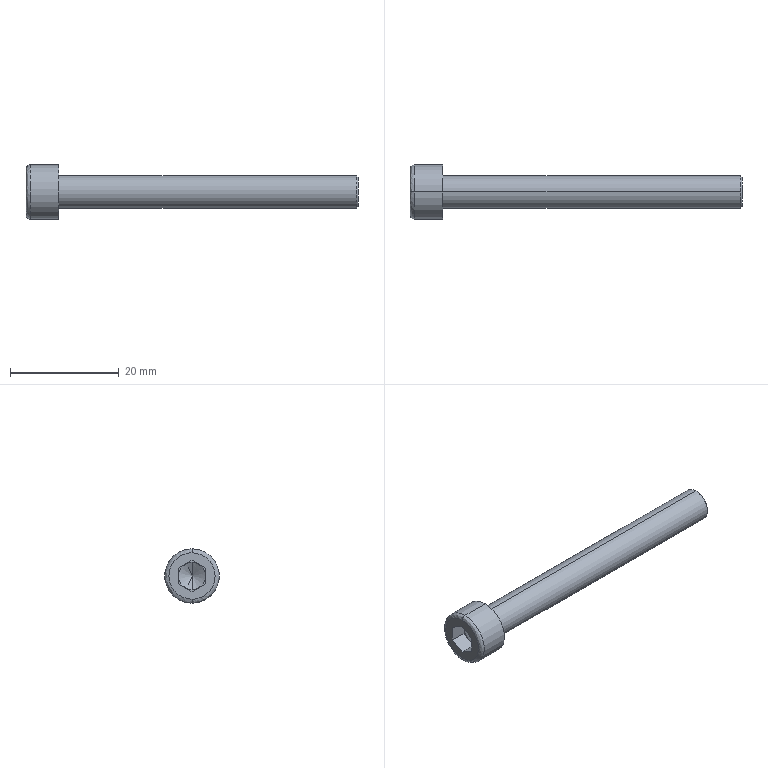Part | STEP file | hexagon socket head cap screws gb_GB_FASTENER_SCREWS_HSHCS M6X55-N | 1 solid | 25 faces | box 61 x 10 x 10 mm | volume 1948 mm3 | plane 15 | cylinder 4 | cone 4 | spline 2 | commonest cylinder face diameters 6 x2 10 x2
STEP:
#1=CARTESIAN_POINT('',(0.75,0.,5.));
#2=VERTEX_POINT('',#1);
#3=CARTESIAN_POINT('',(0.75,0.,-5.));
#4=VERTEX_POINT('',#3);
#5=CARTESIAN_POINT('',(0.75,0.,0.));
#6=DIRECTION('',(1.,0.,0.));
#7=DIRECTION('',(0.,0.,1.));
#8=AXIS2_PLACEMENT_3D('',#5,#6,#7);
#9=CIRCLE('',#8,5.);
#10=EDGE_CURVE('',#2,#4,#9,.T.);
#11=ORIENTED_EDGE('',*,*,#10,.F.);
#12=CARTESIAN_POINT('',(0.,0.,4.25));
#13=VERTEX_POINT('',#12);
#14=CARTESIAN_POINT('',(0.75,0.,4.25));
#15=DIRECTION('',(0.,-1.,0.));
#16=DIRECTION('',(0.,0.,1.));
#17=AXIS2_PLACEMENT_3D('',#14,#15,#16);
#18=CIRCLE('',#17,0.75);
#19=EDGE_CURVE('',#2,#13,#18,.T.);
#20=ORIENTED_EDGE('',*,*,#19,.T.);
#21=CARTESIAN_POINT('',(0.,0.,-4.25));
#22=VERTEX_POINT('',#21);
#23=CARTESIAN_POINT('',(0.,0.,4.25));
#24=CARTESIAN_POINT('',(0.,-8.5,4.25));
#25=CARTESIAN_POINT('',(0.,-8.5,-4.25));
#26=CARTESIAN_POINT('',(0.,0.,-4.25));
#27=(BOUNDED_CURVE()B_SPLINE_CURVE(3,(#23,#24,#25,#26),.UNSPECIFIED.,.F.,.F.)B_SPLINE_CURVE_WITH_KNOTS((4,4),(0.,1.),.UNSPECIFIED.)CURVE()GEOMETRIC_REPRESENTATION_ITEM()RATIONAL_B_SPLINE_CURVE((1.,0.3333,0.3333,1.))REPRESENTATION_ITEM(''));
#28=EDGE_CURVE('',#13,#22,#27,.T.);
#29=ORIENTED_EDGE('',*,*,#28,.T.);
#30=CARTESIAN_POINT('',(0.75,0.,-4.25));
#31=DIRECTION('',(0.,1.,0.));
#32=DIRECTION('',(0.,0.,-1.));
#33=AXIS2_PLACEMENT_3D('',#30,#31,#32);
#34=CIRCLE('',#33,0.75);
#35=EDGE_CURVE('',#4,#22,#34,.T.);
#36=ORIENTED_EDGE('',*,*,#35,.F.);
#37=EDGE_LOOP('',(#11,#20,#29,#36));
#38=FACE_OUTER_BOUND('',#37,.T.);
#39=CARTESIAN_POINT('',(0.75,0.,5.));
#40=CARTESIAN_POINT('',(0.75,-10.,5.));
#41=CARTESIAN_POINT('',(0.75,-10.,-5.));
#42=CARTESIAN_POINT('',(0.75,0.,-5.));
#43=CARTESIAN_POINT('',(0.3107,0.,5.));
#44=CARTESIAN_POINT('',(0.3107,-10.,5.));
#45=CARTESIAN_POINT('',(0.3107,-10.,-5.));
#46=CARTESIAN_POINT('',(0.3107,0.,-5.));
#47=CARTESIAN_POINT('',(0.,0.,4.689));
#48=CARTESIAN_POINT('',(0.,-9.379,4.689));
#49=CARTESIAN_POINT('',(0.,-9.379,-4.689));
#50=CARTESIAN_POINT('',(0.,0.,-4.689));
#51=CARTESIAN_POINT('',(0.,0.,4.25));
#52=CARTESIAN_POINT('',(0.,-8.5,4.25));
#53=CARTESIAN_POINT('',(0.,-8.5,-4.25));
#54=CARTESIAN_POINT('',(0.,0.,-4.25));
#55=(BOUNDED_SURFACE()B_SPLINE_SURFACE(3,3,((#39,#40,#41,#42),(#43,#44,#45,#46),(#47,#48,#49,#50),(#51,#52,#53,#54)),.UNSPECIFIED.,.F.,.F.,.F.)B_SPLINE_SURFACE_WITH_KNOTS((4,4),(4,4),(0.,1.),(0.,1.),.UNSPECIFIED.)GEOMETRIC_REPRESENTATION_ITEM()RATIONAL_B_SPLINE_SURFACE(((1.,0.3333,0.3333,1.),(0.8047,0.2682,0.2682,0.8047),(0.8047,0.2682,0.2682,0.8047),(1.,0.3333,0.3333,1.)))REPRESENTATION_ITEM('')SURFACE());
#56=ADVANCED_FACE('',(#38),#55,.T.);
#57=CARTESIAN_POINT('',(60.75,0.,3.));
#58=VERTEX_POINT('',#57);
#59=CARTESIAN_POINT('',(60.75,0.,-3.));
#60=VERTEX_POINT('',#59);
#61=CARTESIAN_POINT('',(60.75,0.,0.));
#62=DIRECTION('',(-1.,0.,0.));
#63=DIRECTION('',(0.,0.,1.));
#64=AXIS2_PLACEMENT_3D('',#61,#62,#63);
#65=CIRCLE('',#64,3.);
#66=EDGE_CURVE('',#58,#60,#65,.T.);
#67=ORIENTED_EDGE('',*,*,#66,.T.);
#68=CARTESIAN_POINT('',(6.,0.,-3.));
#69=VERTEX_POINT('',#68);
#70=CARTESIAN_POINT('',(61.,0.,-3.));
#71=DIRECTION('',(-1.,0.,0.));
#72=VECTOR('',#71,1000.);
#73=LINE('',#70,#72);
#74=EDGE_CURVE('',#60,#69,#73,.T.);
#75=ORIENTED_EDGE('',*,*,#74,.T.);
#76=CARTESIAN_POINT('',(6.,0.,3.));
#77=VERTEX_POINT('',#76);
#78=CARTESIAN_POINT('',(6.,0.,0.));
#79=DIRECTION('',(1.,0.,0.));
#80=DIRECTION('',(0.,0.,1.));
#81=AXIS2_PLACEMENT_3D('',#78,#79,#80);
#82=CIRCLE('',#81,3.);
#83=EDGE_CURVE('',#69,#77,#82,.T.);
#84=ORIENTED_EDGE('',*,*,#83,.T.);
#85=CARTESIAN_POINT('',(61.,0.,3.));
#86=DIRECTION('',(-1.,0.,0.));
#87=VECTOR('',#86,1000.);
#88=LINE('',#85,#87);
#89=EDGE_CURVE('',#58,#77,#88,.T.);
#90=ORIENTED_EDGE('',*,*,#89,.F.);
#91=EDGE_LOOP('',(#67,#75,#84,#90));
#92=FACE_OUTER_BOUND('',#91,.T.);
#93=CARTESIAN_POINT('',(61.,0.,0.));
#94=DIRECTION('',(-1.,0.,0.));
#95=DIRECTION('',(0.,0.,1.));
#96=AXIS2_PLACEMENT_3D('',#93,#94,#95);
#97=CYLINDRICAL_SURFACE('',#96,3.);
#98=ADVANCED_FACE('',(#92),#97,.T.);
#99=CARTESIAN_POINT('',(61.,0.,2.75));
#100=VERTEX_POINT('',#99);
#101=CARTESIAN_POINT('',(61.,0.,-2.75));
#102=VERTEX_POINT('',#101);
#103=CARTESIAN_POINT('',(61.,0.,0.));
#104=DIRECTION('',(-1.,0.,0.));
#105=DIRECTION('',(0.,0.,1.));
#106=AXIS2_PLACEMENT_3D('',#103,#104,#105);
#107=CIRCLE('',#106,2.75);
#108=EDGE_CURVE('',#100,#102,#107,.T.);
#109=ORIENTED_EDGE('',*,*,#108,.T.);
#110=CARTESIAN_POINT('',(60.75,0.,-3.));
#111=DIRECTION('',(-0.7071,0.,-0.7071));
#112=VECTOR('',#111,1000.);
#113=LINE('',#110,#112);
#114=EDGE_CURVE('',#102,#60,#113,.T.);
#115=ORIENTED_EDGE('',*,*,#114,.T.);
#116=ORIENTED_EDGE('',*,*,#66,.F.);
#117=CARTESIAN_POINT('',(60.75,0.,3.));
#118=DIRECTION('',(-0.7071,0.,0.7071));
#119=VECTOR('',#118,1000.);
#120=LINE('',#117,#119);
#121=EDGE_CURVE('',#100,#58,#120,.T.);
#122=ORIENTED_EDGE('',*,*,#121,.F.);
#123=EDGE_LOOP('',(#109,#115,#116,#122));
#124=FACE_OUTER_BOUND('',#123,.T.);
#125=CARTESIAN_POINT('',(60.75,0.,0.));
#126=DIRECTION('',(-1.,0.,0.));
#127=DIRECTION('',(0.,0.,1.));
#128=AXIS2_PLACEMENT_3D('',#125,#126,#127);
#129=CONICAL_SURFACE('',#128,3.,0.7854);
#130=ADVANCED_FACE('',(#124),#129,.T.);
#131=CARTESIAN_POINT('',(6.,0.,-5.));
#132=VERTEX_POINT('',#131);
#133=CARTESIAN_POINT('',(6.,0.,5.));
#134=VERTEX_POINT('',#133);
#135=CARTESIAN_POINT('',(6.,0.,0.));
#136=DIRECTION('',(1.,0.,0.));
#137=DIRECTION('',(0.,0.,1.));
#138=AXIS2_PLACEMENT_3D('',#135,#136,#137);
#139=CIRCLE('',#138,5.);
#140=EDGE_CURVE('',#132,#134,#139,.T.);
#141=ORIENTED_EDGE('',*,*,#140,.F.);
#142=CARTESIAN_POINT('',(6.,0.,-5.));
#143=DIRECTION('',(-1.,0.,0.));
#144=VECTOR('',#143,1000.);
#145=LINE('',#142,#144);
#146=EDGE_CURVE('',#132,#4,#145,.T.);
#147=ORIENTED_EDGE('',*,*,#146,.T.);
#148=CARTESIAN_POINT('',(0.75,0.,0.));
#149=DIRECTION('',(1.,0.,0.));
#150=DIRECTION('',(0.,0.,1.));
#151=AXIS2_PLACEMENT_3D('',#148,#149,#150);
#152=CIRCLE('',#151,5.);
#153=EDGE_CURVE('',#4,#2,#152,.T.);
#154=ORIENTED_EDGE('',*,*,#153,.T.);
#155=CARTESIAN_POINT('',(6.,0.,5.));
#156=DIRECTION('',(-1.,0.,0.));
#157=VECTOR('',#156,1000.);
#158=LINE('',#155,#157);
#159=EDGE_CURVE('',#134,#2,#158,.T.);
#160=ORIENTED_EDGE('',*,*,#159,.F.);
#161=EDGE_LOOP('',(#141,#147,#154,#160));
#162=FACE_OUTER_BOUND('',#161,.T.);
#163=CARTESIAN_POINT('',(6.,0.,0.));
#164=DIRECTION('',(-1.,0.,0.));
#165=DIRECTION('',(0.,0.,1.));
#166=AXIS2_PLACEMENT_3D('',#163,#164,#165);
#167=CYLINDRICAL_SURFACE('',#166,5.);
#168=ADVANCED_FACE('',(#162),#167,.T.);
#169=CARTESIAN_POINT('',(4.443,0.,0.));
#170=VERTEX_POINT('',#169);
#171=CARTESIAN_POINT('',(3.,0.,2.5));
#172=VERTEX_POINT('',#171);
#173=CARTESIAN_POINT('',(3.,0.,2.5));
#174=DIRECTION('',(-0.5,0.,0.866));
#175=VECTOR('',#174,1000.);
#176=LINE('',#173,#175);
#177=EDGE_CURVE('',#170,#172,#176,.T.);
#178=ORIENTED_EDGE('',*,*,#177,.F.);
#179=CARTESIAN_POINT('',(3.,0.,-2.5));
#180=VERTEX_POINT('',#179);
#181=CARTESIAN_POINT('',(3.,0.,-2.5));
#182=DIRECTION('',(-0.5,0.,-0.866));
#183=VECTOR('',#182,1000.);
#184=LINE('',#181,#183);
#185=EDGE_CURVE('',#170,#180,#184,.T.);
#186=ORIENTED_EDGE('',*,*,#185,.T.);
#187=CARTESIAN_POINT('',(3.,-1.25,-2.165));
#188=VERTEX_POINT('',#187);
#189=CARTESIAN_POINT('',(3.,0.,0.));
#190=DIRECTION('',(1.,0.,0.));
#191=DIRECTION('',(0.,0.,1.));
#192=AXIS2_PLACEMENT_3D('',#189,#190,#191);
#193=CIRCLE('',#192,2.5);
#194=EDGE_CURVE('',#188,#180,#193,.T.);
#195=ORIENTED_EDGE('',*,*,#194,.F.);
#196=CARTESIAN_POINT('',(3.,-2.5,0.));
#197=VERTEX_POINT('',#196);
#198=CARTESIAN_POINT('',(3.,0.,0.));
#199=DIRECTION('',(1.,0.,0.));
#200=DIRECTION('',(0.,0.,1.));
#201=AXIS2_PLACEMENT_3D('',#198,#199,#200);
#202=CIRCLE('',#201,2.5);
#203=EDGE_CURVE('',#197,#188,#202,.T.);
#204=ORIENTED_EDGE('',*,*,#203,.F.);
#205=CARTESIAN_POINT('',(3.,-1.25,2.165));
#206=VERTEX_POINT('',#205);
#207=CARTESIAN_POINT('',(3.,0.,0.));
#208=DIRECTION('',(-1.,0.,0.));
#209=DIRECTION('',(0.,0.,1.));
#210=AXIS2_PLACEMENT_3D('',#207,#208,#209);
#211=CIRCLE('',#210,2.5);
#212=EDGE_CURVE('',#197,#206,#211,.T.);
#213=ORIENTED_EDGE('',*,*,#212,.T.);
#214=CARTESIAN_POINT('',(3.,0.,0.));
#215=DIRECTION('',(1.,0.,0.));
#216=DIRECTION('',(0.,0.,1.));
#217=AXIS2_PLACEMENT_3D('',#214,#215,#216);
#218=CIRCLE('',#217,2.5);
#219=EDGE_CURVE('',#172,#206,#218,.T.);
#220=ORIENTED_EDGE('',*,*,#219,.F.);
#221=EDGE_LOOP('',(#178,#186,#195,#204,#213,#220));
#222=FACE_OUTER_BOUND('',#221,.T.);
#223=CARTESIAN_POINT('',(3.,0.,0.));
#224=DIRECTION('',(-1.,0.,0.));
#225=DIRECTION('',(0.,0.,1.));
#226=AXIS2_PLACEMENT_3D('',#223,#224,#225);
#227=CONICAL_SURFACE('',#226,2.5,1.047);
#228=ADVANCED_FACE('',(#222),#227,.F.);
#229=ORIENTED_EDGE('',*,*,#74,.F.);
#230=CARTESIAN_POINT('',(60.75,0.,0.));
#231=DIRECTION('',(-1.,0.,0.));
#232=DIRECTION('',(0.,0.,1.));
#233=AXIS2_PLACEMENT_3D('',#230,#231,#232);
#234=CIRCLE('',#233,3.);
#235=EDGE_CURVE('',#60,#58,#234,.T.);
#236=ORIENTED_EDGE('',*,*,#235,.T.);
#237=ORIENTED_EDGE('',*,*,#89,.T.);
#238=CARTESIAN_POINT('',(6.,0.,0.));
#239=DIRECTION('',(1.,0.,0.));
#240=DIRECTION('',(0.,0.,1.));
#241=AXIS2_PLACEMENT_3D('',#238,#239,#240);
#242=CIRCLE('',#241,3.);
#243=EDGE_CURVE('',#77,#69,#242,.T.);
#244=ORIENTED_EDGE('',*,*,#243,.T.);
#245=EDGE_LOOP('',(#229,#236,#237,#244));
#246=FACE_OUTER_BOUND('',#245,.T.);
#247=CARTESIAN_POINT('',(61.,0.,0.));
#248=DIRECTION('',(-1.,0.,0.));
#249=DIRECTION('',(0.,0.,1.));
#250=AXIS2_PLACEMENT_3D('',#247,#248,#249);
#251=CYLINDRICAL_SURFACE('',#250,3.);
#252=ADVANCED_FACE('',(#246),#251,.T.);
#253=ORIENTED_EDGE('',*,*,#243,.F.);
#254=ORIENTED_EDGE('',*,*,#83,.F.);
#255=EDGE_LOOP('',(#253,#254));
#256=FACE_BOUND('',#255,.T.);
#257=CARTESIAN_POINT('',(6.,0.,0.));
#258=DIRECTION('',(1.,0.,0.));
#259=DIRECTION('',(0.,0.,1.));
#260=AXIS2_PLACEMENT_3D('',#257,#258,#259);
#261=CIRCLE('',#260,5.);
#262=EDGE_CURVE('',#134,#132,#261,.T.);
#263=ORIENTED_EDGE('',*,*,#262,.T.);
#264=ORIENTED_EDGE('',*,*,#140,.T.);
#265=EDGE_LOOP('',(#263,#264));
#266=FACE_OUTER_BOUND('',#265,.T.);
#267=CARTESIAN_POINT('',(6.,0.,0.));
#268=DIRECTION('',(1.,0.,0.));
#269=DIRECTION('',(0.,0.,-1.));
#270=AXIS2_PLACEMENT_3D('',#267,#268,#269);
#271=PLANE('',#270);
#272=ADVANCED_FACE('',(#256,#266),#271,.T.);
#273=ORIENTED_EDGE('',*,*,#114,.F.);
#274=CARTESIAN_POINT('',(61.,0.,0.));
#275=DIRECTION('',(-1.,0.,0.));
#276=DIRECTION('',(0.,0.,1.));
#277=AXIS2_PLACEMENT_3D('',#274,#275,#276);
#278=CIRCLE('',#277,2.75);
#279=EDGE_CURVE('',#102,#100,#278,.T.);
#280=ORIENTED_EDGE('',*,*,#279,.T.);
#281=ORIENTED_EDGE('',*,*,#121,.T.);
#282=ORIENTED_EDGE('',*,*,#235,.F.);
#283=EDGE_LOOP('',(#273,#280,#281,#282));
#284=FACE_OUTER_BOUND('',#283,.T.);
#285=CARTESIAN_POINT('',(60.75,0.,0.));
#286=DIRECTION('',(-1.,0.,0.));
#287=DIRECTION('',(0.,0.,1.));
#288=AXIS2_PLACEMENT_3D('',#285,#286,#287);
#289=CONICAL_SURFACE('',#288,3.,0.7854);
#290=ADVANCED_FACE('',(#284),#289,.T.);
#291=ORIENTED_EDGE('',*,*,#146,.F.);
#292=ORIENTED_EDGE('',*,*,#262,.F.);
#293=ORIENTED_EDGE('',*,*,#159,.T.);
#294=ORIENTED_EDGE('',*,*,#10,.T.);
#295=EDGE_LOOP('',(#291,#292,#293,#294));
#296=FACE_OUTER_BOUND('',#295,.T.);
#297=CARTESIAN_POINT('',(6.,0.,0.));
#298=DIRECTION('',(-1.,0.,0.));
#299=DIRECTION('',(0.,0.,1.));
#300=AXIS2_PLACEMENT_3D('',#297,#298,#299);
#301=CYLINDRICAL_SURFACE('',#300,5.);
#302=ADVANCED_FACE('',(#296),#301,.T.);
#303=ORIENTED_EDGE('',*,*,#108,.F.);
#304=ORIENTED_EDGE('',*,*,#279,.F.);
#305=EDGE_LOOP('',(#303,#304));
#306=FACE_OUTER_BOUND('',#305,.T.);
#307=CARTESIAN_POINT('',(61.,0.,0.));
#308=DIRECTION('',(1.,0.,0.));
#309=DIRECTION('',(0.,0.,-1.));
#310=AXIS2_PLACEMENT_3D('',#307,#308,#309);
#311=PLANE('',#310);
#312=ADVANCED_FACE('',(#306),#311,.T.);
#313=ORIENTED_EDGE('',*,*,#19,.F.);
#314=ORIENTED_EDGE('',*,*,#153,.F.);
#315=ORIENTED_EDGE('',*,*,#35,.T.);
#316=CARTESIAN_POINT('',(0.,0.,-4.25));
#317=CARTESIAN_POINT('',(0.,8.5,-4.25));
#318=CARTESIAN_POINT('',(0.,8.5,4.25));
#319=CARTESIAN_POINT('',(0.,0.,4.25));
#320=(BOUNDED_CURVE()B_SPLINE_CURVE(3,(#316,#317,#318,#319),.UNSPECIFIED.,.F.,.T.)B_SPLINE_CURVE_WITH_KNOTS((4,4),(0.,1.),.UNSPECIFIED.)CURVE()GEOMETRIC_REPRESENTATION_ITEM()RATIONAL_B_SPLINE_CURVE((1.,0.3333,0.3333,1.))REPRESENTATION_ITEM(''));
#321=EDGE_CURVE('',#22,#13,#320,.T.);
#322=ORIENTED_EDGE('',*,*,#321,.T.);
#323=EDGE_LOOP('',(#313,#314,#315,#322));
#324=FACE_OUTER_BOUND('',#323,.T.);
#325=CARTESIAN_POINT('',(0.75,0.,-5.));
#326=CARTESIAN_POINT('',(0.75,10.,-5.));
#327=CARTESIAN_POINT('',(0.75,10.,5.));
#328=CARTESIAN_POINT('',(0.75,0.,5.));
#329=CARTESIAN_POINT('',(0.3107,0.,-5.));
#330=CARTESIAN_POINT('',(0.3107,10.,-5.));
#331=CARTESIAN_POINT('',(0.3107,10.,5.));
#332=CARTESIAN_POINT('',(0.3107,0.,5.));
#333=CARTESIAN_POINT('',(0.,0.,-4.689));
#334=CARTESIAN_POINT('',(0.,9.379,-4.689));
#335=CARTESIAN_POINT('',(0.,9.379,4.689));
#336=CARTESIAN_POINT('',(0.,0.,4.689));
#337=CARTESIAN_POINT('',(0.,0.,-4.25));
#338=CARTESIAN_POINT('',(0.,8.5,-4.25));
#339=CARTESIAN_POINT('',(0.,8.5,4.25));
#340=CARTESIAN_POINT('',(0.,0.,4.25));
#341=(BOUNDED_SURFACE()B_SPLINE_SURFACE(3,3,((#325,#326,#327,#328),(#329,#330,#331,#332),(#333,#334,#335,#336),(#337,#338,#339,#340)),.UNSPECIFIED.,.F.,.F.,.F.)B_SPLINE_SURFACE_WITH_KNOTS((4,4),(4,4),(0.,1.),(0.,1.),.UNSPECIFIED.)GEOMETRIC_REPRESENTATION_ITEM()RATIONAL_B_SPLINE_SURFACE(((1.,0.3333,0.3333,1.),(0.8047,0.2682,0.2682,0.8047),(0.8047,0.2682,0.2682,0.8047),(1.,0.3333,0.3333,1.)))REPRESENTATION_ITEM('')SURFACE());
#342=ADVANCED_FACE('',(#324),#341,.T.);
#343=CARTESIAN_POINT('',(0.,2.5,-1.443));
#344=VERTEX_POINT('',#343);
#345=CARTESIAN_POINT('',(0.,0.,-2.887));
#346=VERTEX_POINT('',#345);
#347=CARTESIAN_POINT('',(0.,2.5,-1.443));
#348=DIRECTION('',(0.,-0.866,-0.5));
#349=VECTOR('',#348,1000.);
#350=LINE('',#347,#349);
#351=EDGE_CURVE('',#344,#346,#350,.T.);
#352=ORIENTED_EDGE('',*,*,#351,.F.);
#353=CARTESIAN_POINT('',(0.,2.5,1.443));
#354=VERTEX_POINT('',#353);
#355=CARTESIAN_POINT('',(0.,2.5,0.));
#356=DIRECTION('',(0.,0.,-1.));
#357=VECTOR('',#356,1000.);
#358=LINE('',#355,#357);
#359=EDGE_CURVE('',#354,#344,#358,.T.);
#360=ORIENTED_EDGE('',*,*,#359,.F.);
#361=CARTESIAN_POINT('',(0.,0.,2.887));
#362=VERTEX_POINT('',#361);
#363=CARTESIAN_POINT('',(0.,0.,2.887));
#364=DIRECTION('',(0.,0.866,-0.5));
#365=VECTOR('',#364,1000.);
#366=LINE('',#363,#365);
#367=EDGE_CURVE('',#362,#354,#366,.T.);
#368=ORIENTED_EDGE('',*,*,#367,.F.);
#369=CARTESIAN_POINT('',(0.,-2.5,1.443));
#370=VERTEX_POINT('',#369);
#371=CARTESIAN_POINT('',(0.,-2.5,1.443));
#372=DIRECTION('',(0.,0.866,0.5));
#373=VECTOR('',#372,1000.);
#374=LINE('',#371,#373);
#375=EDGE_CURVE('',#370,#362,#374,.T.);
#376=ORIENTED_EDGE('',*,*,#375,.F.);
#377=CARTESIAN_POINT('',(0.,-2.5,-1.443));
#378=VERTEX_POINT('',#377);
#379=CARTESIAN_POINT('',(0.,-2.5,0.));
#380=DIRECTION('',(0.,0.,1.));
#381=VECTOR('',#380,1000.);
#382=LINE('',#379,#381);
#383=EDGE_CURVE('',#378,#370,#382,.T.);
#384=ORIENTED_EDGE('',*,*,#383,.F.);
#385=CARTESIAN_POINT('',(0.,0.,-2.887));
#386=DIRECTION('',(0.,-0.866,0.5));
#387=VECTOR('',#386,1000.);
#388=LINE('',#385,#387);
#389=EDGE_CURVE('',#346,#378,#388,.T.);
#390=ORIENTED_EDGE('',*,*,#389,.F.);
#391=EDGE_LOOP('',(#352,#360,#368,#376,#384,#390));
#392=FACE_BOUND('',#391,.T.);
#393=ORIENTED_EDGE('',*,*,#321,.F.);
#394=ORIENTED_EDGE('',*,*,#28,.F.);
#395=EDGE_LOOP('',(#393,#394));
#396=FACE_OUTER_BOUND('',#395,.T.);
#397=CARTESIAN_POINT('',(0.,0.,0.));
#398=DIRECTION('',(1.,0.,0.));
#399=DIRECTION('',(0.,0.,-1.));
#400=AXIS2_PLACEMENT_3D('',#397,#398,#399);
#401=PLANE('',#400);
#402=ADVANCED_FACE('',(#392,#396),#401,.F.);
#403=CARTESIAN_POINT('',(3.,0.,-2.887));
#404=VERTEX_POINT('',#403);
#405=CARTESIAN_POINT('',(3.,-2.5,-1.443));
#406=DIRECTION('',(0.,0.866,-0.5));
#407=VECTOR('',#406,1000.);
#408=LINE('',#405,#407);
#409=EDGE_CURVE('',#188,#404,#408,.T.);
#410=ORIENTED_EDGE('',*,*,#409,.T.);
#411=CARTESIAN_POINT('',(3.,0.,-2.887));
#412=DIRECTION('',(-1.,0.,0.));
#413=VECTOR('',#412,1000.);
#414=LINE('',#411,#413);
#415=EDGE_CURVE('',#404,#346,#414,.T.);
#416=ORIENTED_EDGE('',*,*,#415,.T.);
#417=ORIENTED_EDGE('',*,*,#389,.T.);
#418=CARTESIAN_POINT('',(3.,-2.5,-1.443));
#419=VERTEX_POINT('',#418);
#420=CARTESIAN_POINT('',(3.,-2.5,-1.443));
#421=DIRECTION('',(1.,0.,0.));
#422=VECTOR('',#421,1000.);
#423=LINE('',#420,#422);
#424=EDGE_CURVE('',#378,#419,#423,.T.);
#425=ORIENTED_EDGE('',*,*,#424,.T.);
#426=CARTESIAN_POINT('',(3.,-2.5,-1.443));
#427=DIRECTION('',(0.,0.866,-0.5));
#428=VECTOR('',#427,1000.);
#429=LINE('',#426,#428);
#430=EDGE_CURVE('',#419,#188,#429,.T.);
#431=ORIENTED_EDGE('',*,*,#430,.T.);
#432=EDGE_LOOP('',(#410,#416,#417,#425,#431));
#433=FACE_OUTER_BOUND('',#432,.T.);
#434=CARTESIAN_POINT('',(3.,-2.5,-1.443));
#435=DIRECTION('',(0.,0.5,0.866));
#436=DIRECTION('',(0.,-0.866,0.5));
#437=AXIS2_PLACEMENT_3D('',#434,#435,#436);
#438=PLANE('',#437);
#439=ADVANCED_FACE('',(#433),#438,.T.);
#440=CARTESIAN_POINT('',(3.,1.25,-2.165));
#441=VERTEX_POINT('',#440);
#442=CARTESIAN_POINT('',(3.,2.5,-1.443));
#443=VERTEX_POINT('',#442);
#444=CARTESIAN_POINT('',(3.,1.25,-2.165));
#445=DIRECTION('',(0.,0.866,0.5));
#446=VECTOR('',#445,1000.);
#447=LINE('',#444,#446);
#448=EDGE_CURVE('',#441,#443,#447,.T.);
#449=ORIENTED_EDGE('',*,*,#448,.T.);
#450=CARTESIAN_POINT('',(3.,2.5,-1.443));
#451=DIRECTION('',(-1.,0.,0.));
#452=VECTOR('',#451,1000.);
#453=LINE('',#450,#452);
#454=EDGE_CURVE('',#443,#344,#453,.T.);
#455=ORIENTED_EDGE('',*,*,#454,.T.);
#456=ORIENTED_EDGE('',*,*,#351,.T.);
#457=ORIENTED_EDGE('',*,*,#415,.F.);
#458=CARTESIAN_POINT('',(3.,0.,-2.887));
#459=DIRECTION('',(0.,0.866,0.5));
#460=VECTOR('',#459,1000.);
#461=LINE('',#458,#460);
#462=EDGE_CURVE('',#404,#441,#461,.T.);
#463=ORIENTED_EDGE('',*,*,#462,.T.);
#464=EDGE_LOOP('',(#449,#455,#456,#457,#463));
#465=FACE_OUTER_BOUND('',#464,.T.);
#466=CARTESIAN_POINT('',(3.,0.,-2.887));
#467=DIRECTION('',(0.,-0.5,0.866));
#468=DIRECTION('',(0.,-0.866,-0.5));
#469=AXIS2_PLACEMENT_3D('',#466,#467,#468);
#470=PLANE('',#469);
#471=ADVANCED_FACE('',(#465),#470,.T.);
#472=CARTESIAN_POINT('',(3.,2.5,0.));
#473=VERTEX_POINT('',#472);
#474=CARTESIAN_POINT('',(3.,2.5,1.443));
#475=VERTEX_POINT('',#474);
#476=CARTESIAN_POINT('',(3.,2.5,-2.887));
#477=DIRECTION('',(0.,0.,1.));
#478=VECTOR('',#477,1000.);
#479=LINE('',#476,#478);
#480=EDGE_CURVE('',#473,#475,#479,.T.);
#481=ORIENTED_EDGE('',*,*,#480,.T.);
#482=CARTESIAN_POINT('',(3.,2.5,1.443));
#483=DIRECTION('',(-1.,0.,0.));
#484=VECTOR('',#483,1000.);
#485=LINE('',#482,#484);
#486=EDGE_CURVE('',#475,#354,#485,.T.);
#487=ORIENTED_EDGE('',*,*,#486,.T.);
#488=ORIENTED_EDGE('',*,*,#359,.T.);
#489=ORIENTED_EDGE('',*,*,#454,.F.);
#490=CARTESIAN_POINT('',(3.,2.5,-2.887));
#491=DIRECTION('',(0.,0.,1.));
#492=VECTOR('',#491,1000.);
#493=LINE('',#490,#492);
#494=EDGE_CURVE('',#443,#473,#493,.T.);
#495=ORIENTED_EDGE('',*,*,#494,.T.);
#496=EDGE_LOOP('',(#481,#487,#488,#489,#495));
#497=FACE_OUTER_BOUND('',#496,.T.);
#498=CARTESIAN_POINT('',(3.,2.5,-1.443));
#499=DIRECTION('',(0.,-1.,0.));
#500=DIRECTION('',(0.,0.,-1.));
#501=AXIS2_PLACEMENT_3D('',#498,#499,#500);
#502=PLANE('',#501);
#503=ADVANCED_FACE('',(#497),#502,.T.);
#504=CARTESIAN_POINT('',(3.,1.25,2.165));
#505=VERTEX_POINT('',#504);
#506=CARTESIAN_POINT('',(3.,0.,2.887));
#507=VERTEX_POINT('',#506);
#508=CARTESIAN_POINT('',(3.,2.5,1.443));
#509=DIRECTION('',(0.,-0.866,0.5));
#510=VECTOR('',#509,1000.);
#511=LINE('',#508,#510);
#512=EDGE_CURVE('',#505,#507,#511,.T.);
#513=ORIENTED_EDGE('',*,*,#512,.T.);
#514=CARTESIAN_POINT('',(3.,0.,2.887));
#515=DIRECTION('',(-1.,0.,0.));
#516=VECTOR('',#515,1000.);
#517=LINE('',#514,#516);
#518=EDGE_CURVE('',#507,#362,#517,.T.);
#519=ORIENTED_EDGE('',*,*,#518,.T.);
#520=ORIENTED_EDGE('',*,*,#367,.T.);
#521=ORIENTED_EDGE('',*,*,#486,.F.);
#522=CARTESIAN_POINT('',(3.,2.5,1.443));
#523=DIRECTION('',(0.,-0.866,0.5));
#524=VECTOR('',#523,1000.);
#525=LINE('',#522,#524);
#526=EDGE_CURVE('',#475,#505,#525,.T.);
#527=ORIENTED_EDGE('',*,*,#526,.T.);
#528=EDGE_LOOP('',(#513,#519,#520,#521,#527));
#529=FACE_OUTER_BOUND('',#528,.T.);
#530=CARTESIAN_POINT('',(3.,2.5,1.443));
#531=DIRECTION('',(0.,-0.5,-0.866));
#532=DIRECTION('',(0.,0.866,-0.5));
#533=AXIS2_PLACEMENT_3D('',#530,#531,#532);
#534=PLANE('',#533);
#535=ADVANCED_FACE('',(#529),#534,.T.);
#536=CARTESIAN_POINT('',(3.,-2.5,1.443));
#537=VERTEX_POINT('',#536);
#538=CARTESIAN_POINT('',(3.,0.,2.887));
#539=DIRECTION('',(0.,-0.866,-0.5));
#540=VECTOR('',#539,1000.);
#541=LINE('',#538,#540);
#542=EDGE_CURVE('',#206,#537,#541,.T.);
#543=ORIENTED_EDGE('',*,*,#542,.T.);
#544=CARTESIAN_POINT('',(3.,-2.5,1.443));
#545=DIRECTION('',(-1.,0.,0.));
#546=VECTOR('',#545,1000.);
#547=LINE('',#544,#546);
#548=EDGE_CURVE('',#537,#370,#547,.T.);
#549=ORIENTED_EDGE('',*,*,#548,.T.);
#550=ORIENTED_EDGE('',*,*,#375,.T.);
#551=ORIENTED_EDGE('',*,*,#518,.F.);
#552=CARTESIAN_POINT('',(3.,0.,2.887));
#553=DIRECTION('',(0.,-0.866,-0.5));
#554=VECTOR('',#553,1000.);
#555=LINE('',#552,#554);
#556=EDGE_CURVE('',#507,#206,#555,.T.);
#557=ORIENTED_EDGE('',*,*,#556,.T.);
#558=EDGE_LOOP('',(#543,#549,#550,#551,#557));
#559=FACE_OUTER_BOUND('',#558,.T.);
#560=CARTESIAN_POINT('',(3.,0.,2.887));
#561=DIRECTION('',(0.,0.5,-0.866));
#562=DIRECTION('',(0.,0.866,0.5));
#563=AXIS2_PLACEMENT_3D('',#560,#561,#562);
#564=PLANE('',#563);
#565=ADVANCED_FACE('',(#559),#564,.T.);
#566=CARTESIAN_POINT('',(3.,-2.5,-2.887));
#567=DIRECTION('',(0.,0.,-1.));
#568=VECTOR('',#567,1000.);
#569=LINE('',#566,#568);
#570=EDGE_CURVE('',#197,#419,#569,.T.);
#571=ORIENTED_EDGE('',*,*,#570,.T.);
#572=ORIENTED_EDGE('',*,*,#424,.F.);
#573=ORIENTED_EDGE('',*,*,#383,.T.);
#574=ORIENTED_EDGE('',*,*,#548,.F.);
#575=CARTESIAN_POINT('',(3.,-2.5,1.443));
#576=DIRECTION('',(0.,0.,-1.));
#577=VECTOR('',#576,1000.);
#578=LINE('',#575,#577);
#579=EDGE_CURVE('',#537,#197,#578,.T.);
#580=ORIENTED_EDGE('',*,*,#579,.T.);
#581=EDGE_LOOP('',(#571,#572,#573,#574,#580));
#582=FACE_OUTER_BOUND('',#581,.T.);
#583=CARTESIAN_POINT('',(3.,-2.5,1.443));
#584=DIRECTION('',(0.,1.,0.));
#585=DIRECTION('',(0.,0.,1.));
#586=AXIS2_PLACEMENT_3D('',#583,#584,#585);
#587=PLANE('',#586);
#588=ADVANCED_FACE('',(#582),#587,.T.);
#589=ORIENTED_EDGE('',*,*,#462,.F.);
#590=ORIENTED_EDGE('',*,*,#409,.F.);
#591=ORIENTED_EDGE('',*,*,#194,.T.);
#592=CARTESIAN_POINT('',(3.,0.,0.));
#593=DIRECTION('',(1.,0.,0.));
#594=DIRECTION('',(0.,0.,1.));
#595=AXIS2_PLACEMENT_3D('',#592,#593,#594);
#596=CIRCLE('',#595,2.5);
#597=EDGE_CURVE('',#180,#441,#596,.T.);
#598=ORIENTED_EDGE('',*,*,#597,.T.);
#599=EDGE_LOOP('',(#589,#590,#591,#598));
#600=FACE_OUTER_BOUND('',#599,.T.);
#601=CARTESIAN_POINT('',(3.,0.,-2.887));
#602=DIRECTION('',(1.,0.,0.));
#603=DIRECTION('',(0.,0.,-1.));
#604=AXIS2_PLACEMENT_3D('',#601,#602,#603);
#605=PLANE('',#604);
#606=ADVANCED_FACE('',(#600),#605,.F.);
#607=ORIENTED_EDGE('',*,*,#556,.F.);
#608=ORIENTED_EDGE('',*,*,#512,.F.);
#609=CARTESIAN_POINT('',(3.,0.,0.));
#610=DIRECTION('',(1.,0.,0.));
#611=DIRECTION('',(0.,0.,1.));
#612=AXIS2_PLACEMENT_3D('',#609,#610,#611);
#613=CIRCLE('',#612,2.5);
#614=EDGE_CURVE('',#505,#172,#613,.T.);
#615=ORIENTED_EDGE('',*,*,#614,.T.);
#616=ORIENTED_EDGE('',*,*,#219,.T.);
#617=EDGE_LOOP('',(#607,#608,#615,#616));
#618=FACE_OUTER_BOUND('',#617,.T.);
#619=CARTESIAN_POINT('',(3.,0.,-2.887));
#620=DIRECTION('',(1.,0.,0.));
#621=DIRECTION('',(0.,0.,-1.));
#622=AXIS2_PLACEMENT_3D('',#619,#620,#621);
#623=PLANE('',#622);
#624=ADVANCED_FACE('',(#618),#623,.F.);
#625=ORIENTED_EDGE('',*,*,#579,.F.);
#626=ORIENTED_EDGE('',*,*,#542,.F.);
#627=ORIENTED_EDGE('',*,*,#212,.F.);
#628=EDGE_LOOP('',(#625,#626,#627));
#629=FACE_OUTER_BOUND('',#628,.T.);
#630=CARTESIAN_POINT('',(3.,0.,-2.887));
#631=DIRECTION('',(1.,0.,0.));
#632=DIRECTION('',(0.,0.,-1.));
#633=AXIS2_PLACEMENT_3D('',#630,#631,#632);
#634=PLANE('',#633);
#635=ADVANCED_FACE('',(#629),#634,.F.);
#636=ORIENTED_EDGE('',*,*,#185,.F.);
#637=ORIENTED_EDGE('',*,*,#177,.T.);
#638=ORIENTED_EDGE('',*,*,#614,.F.);
#639=CARTESIAN_POINT('',(3.,0.,0.));
#640=DIRECTION('',(1.,0.,0.));
#641=DIRECTION('',(0.,0.,1.));
#642=AXIS2_PLACEMENT_3D('',#639,#640,#641);
#643=CIRCLE('',#642,2.5);
#644=EDGE_CURVE('',#473,#505,#643,.T.);
#645=ORIENTED_EDGE('',*,*,#644,.F.);
#646=CARTESIAN_POINT('',(3.,0.,0.));
#647=DIRECTION('',(1.,0.,0.));
#648=DIRECTION('',(0.,0.,1.));
#649=AXIS2_PLACEMENT_3D('',#646,#647,#648);
#650=CIRCLE('',#649,2.5);
#651=EDGE_CURVE('',#441,#473,#650,.T.);
#652=ORIENTED_EDGE('',*,*,#651,.F.);
#653=ORIENTED_EDGE('',*,*,#597,.F.);
#654=EDGE_LOOP('',(#636,#637,#638,#645,#652,#653));
#655=FACE_OUTER_BOUND('',#654,.T.);
#656=CARTESIAN_POINT('',(3.,0.,0.));
#657=DIRECTION('',(-1.,0.,0.));
#658=DIRECTION('',(0.,0.,1.));
#659=AXIS2_PLACEMENT_3D('',#656,#657,#658);
#660=CONICAL_SURFACE('',#659,2.5,1.047);
#661=ADVANCED_FACE('',(#655),#660,.F.);
#662=ORIENTED_EDGE('',*,*,#430,.F.);
#663=ORIENTED_EDGE('',*,*,#570,.F.);
#664=ORIENTED_EDGE('',*,*,#203,.T.);
#665=EDGE_LOOP('',(#662,#663,#664));
#666=FACE_OUTER_BOUND('',#665,.T.);
#667=CARTESIAN_POINT('',(3.,0.,-2.887));
#668=DIRECTION('',(1.,0.,0.));
#669=DIRECTION('',(0.,0.,-1.));
#670=AXIS2_PLACEMENT_3D('',#667,#668,#669);
#671=PLANE('',#670);
#672=ADVANCED_FACE('',(#666),#671,.F.);
#673=ORIENTED_EDGE('',*,*,#526,.F.);
#674=ORIENTED_EDGE('',*,*,#480,.F.);
#675=ORIENTED_EDGE('',*,*,#644,.T.);
#676=EDGE_LOOP('',(#673,#674,#675));
#677=FACE_OUTER_BOUND('',#676,.T.);
#678=CARTESIAN_POINT('',(3.,0.,-2.887));
#679=DIRECTION('',(1.,0.,0.));
#680=DIRECTION('',(0.,0.,-1.));
#681=AXIS2_PLACEMENT_3D('',#678,#679,#680);
#682=PLANE('',#681);
#683=ADVANCED_FACE('',(#677),#682,.F.);
#684=ORIENTED_EDGE('',*,*,#494,.F.);
#685=ORIENTED_EDGE('',*,*,#448,.F.);
#686=ORIENTED_EDGE('',*,*,#651,.T.);
#687=EDGE_LOOP('',(#684,#685,#686));
#688=FACE_OUTER_BOUND('',#687,.T.);
#689=CARTESIAN_POINT('',(3.,0.,-2.887));
#690=DIRECTION('',(1.,0.,0.));
#691=DIRECTION('',(0.,0.,-1.));
#692=AXIS2_PLACEMENT_3D('',#689,#690,#691);
#693=PLANE('',#692);
#694=ADVANCED_FACE('',(#688),#693,.F.);
#695=CLOSED_SHELL('',(#56,#98,#130,#168,#228,#252,#272,#290,#302,#312,#342,#402,#439,#471,#503,#535,#565,#588,#606,#624,#635,#661,#672,#683,#694));
#696=MANIFOLD_SOLID_BREP('',#695);
#697=CARTESIAN_POINT('',(0.,0.,0.));
#698=DIRECTION('',(0.,0.,1.));
#699=DIRECTION('',(1.,0.,0.));
#700=AXIS2_PLACEMENT_3D('',#697,#698,#699);
#701=(LENGTH_UNIT()NAMED_UNIT(*)SI_UNIT(.MILLI.,.METRE.));
#702=UNCERTAINTY_MEASURE_WITH_UNIT(LENGTH_MEASURE(0.00001),#701,'','');
#703=(NAMED_UNIT(*)PLANE_ANGLE_UNIT()SI_UNIT($,.RADIAN.));
#704=(NAMED_UNIT(*)SI_UNIT($,.STERADIAN.)SOLID_ANGLE_UNIT());
#705=(GEOMETRIC_REPRESENTATION_CONTEXT(3)GLOBAL_UNCERTAINTY_ASSIGNED_CONTEXT((#702))GLOBAL_UNIT_ASSIGNED_CONTEXT((#701,#703,#704))REPRESENTATION_CONTEXT('',''));
#706=ADVANCED_BREP_SHAPE_REPRESENTATION('',(#696,#700),#705);